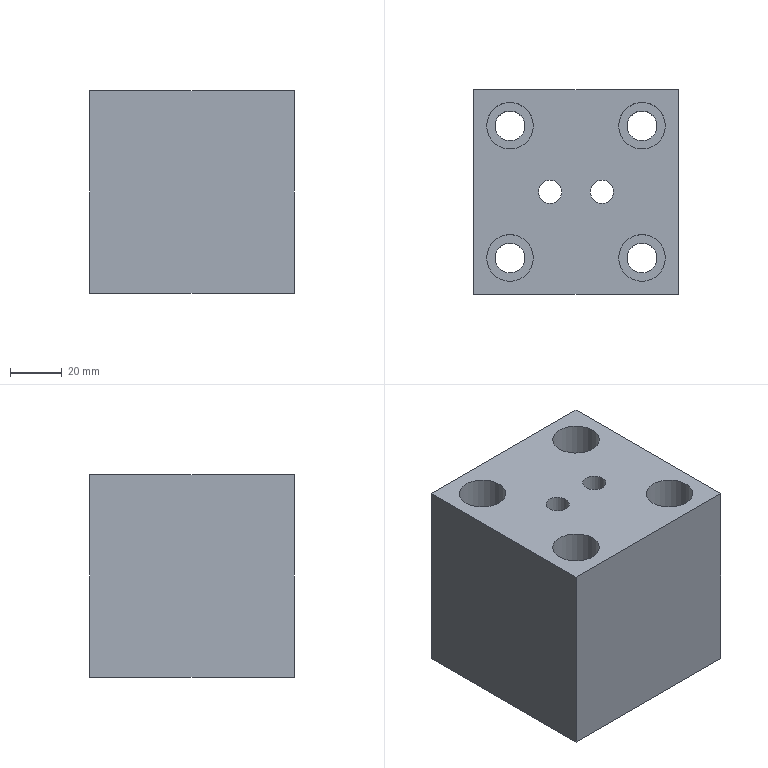Part | STEP file | lll_id4366_x_t | 1 solid | 24 faces | box 79 x 79 x 78 mm | volume 421284 mm3 | plane 12 | cylinder 12 | commonest cylinder face diameters 11.509 x4 18.008 x4 9 x2 14 x2
STEP:
#1=CARTESIAN_POINT('',(2491.255,144.5,-370.));
#2=VERTEX_POINT('',#1);
#3=CARTESIAN_POINT('',(2485.5,144.5,-370.));
#4=DIRECTION('',(0.,0.,1.));
#5=DIRECTION('',(1.,0.,0.));
#6=AXIS2_PLACEMENT_3D('',#3,#4,#5);
#7=CIRCLE('',#6,5.755);
#8=EDGE_CURVE('',#2,#2,#7,.T.);
#9=ORIENTED_EDGE('',*,*,#8,.T.);
#10=EDGE_LOOP('',(#9));
#11=FACE_BOUND('',#10,.T.);
#12=CARTESIAN_POINT('',(2491.255,195.5,-370.));
#13=VERTEX_POINT('',#12);
#14=CARTESIAN_POINT('',(2485.5,195.5,-370.));
#15=DIRECTION('',(0.,0.,1.));
#16=DIRECTION('',(1.,0.,0.));
#17=AXIS2_PLACEMENT_3D('',#14,#15,#16);
#18=CIRCLE('',#17,5.755);
#19=EDGE_CURVE('',#13,#13,#18,.T.);
#20=ORIENTED_EDGE('',*,*,#19,.T.);
#21=EDGE_LOOP('',(#20));
#22=FACE_BOUND('',#21,.T.);
#23=CARTESIAN_POINT('',(2440.255,144.5,-370.));
#24=VERTEX_POINT('',#23);
#25=CARTESIAN_POINT('',(2434.5,144.5,-370.));
#26=DIRECTION('',(0.,0.,1.));
#27=DIRECTION('',(1.,0.,0.));
#28=AXIS2_PLACEMENT_3D('',#25,#26,#27);
#29=CIRCLE('',#28,5.755);
#30=EDGE_CURVE('',#24,#24,#29,.T.);
#31=ORIENTED_EDGE('',*,*,#30,.T.);
#32=EDGE_LOOP('',(#31));
#33=FACE_BOUND('',#32,.T.);
#34=CARTESIAN_POINT('',(2440.255,195.5,-370.));
#35=VERTEX_POINT('',#34);
#36=CARTESIAN_POINT('',(2434.5,195.5,-370.));
#37=DIRECTION('',(0.,0.,1.));
#38=DIRECTION('',(1.,0.,0.));
#39=AXIS2_PLACEMENT_3D('',#36,#37,#38);
#40=CIRCLE('',#39,5.755);
#41=EDGE_CURVE('',#35,#35,#40,.T.);
#42=ORIENTED_EDGE('',*,*,#41,.T.);
#43=EDGE_LOOP('',(#42));
#44=FACE_BOUND('',#43,.T.);
#45=CARTESIAN_POINT('',(2499.5,130.5,-370.));
#46=VERTEX_POINT('',#45);
#47=CARTESIAN_POINT('',(2499.5,209.5,-370.));
#48=VERTEX_POINT('',#47);
#49=CARTESIAN_POINT('',(2499.5,477.5,-370.));
#50=DIRECTION('',(0.,1.,0.));
#51=VECTOR('',#50,1.);
#52=LINE('',#49,#51);
#53=EDGE_CURVE('',#46,#48,#52,.T.);
#54=ORIENTED_EDGE('',*,*,#53,.F.);
#55=CARTESIAN_POINT('',(2420.5,130.5,-370.));
#56=VERTEX_POINT('',#55);
#57=CARTESIAN_POINT('',(2460.,130.5,-370.));
#58=DIRECTION('',(-1.,0.,0.));
#59=VECTOR('',#58,1.);
#60=LINE('',#57,#59);
#61=EDGE_CURVE('',#46,#56,#60,.T.);
#62=ORIENTED_EDGE('',*,*,#61,.T.);
#63=CARTESIAN_POINT('',(2420.5,209.5,-370.));
#64=VERTEX_POINT('',#63);
#65=CARTESIAN_POINT('',(2420.5,477.5,-370.));
#66=DIRECTION('',(0.,-1.,0.));
#67=VECTOR('',#66,1.);
#68=LINE('',#65,#67);
#69=EDGE_CURVE('',#64,#56,#68,.T.);
#70=ORIENTED_EDGE('',*,*,#69,.F.);
#71=CARTESIAN_POINT('',(3042.,209.5,-370.));
#72=DIRECTION('',(-1.,0.,0.));
#73=VECTOR('',#72,1.);
#74=LINE('',#71,#73);
#75=EDGE_CURVE('',#48,#64,#74,.T.);
#76=ORIENTED_EDGE('',*,*,#75,.F.);
#77=EDGE_LOOP('',(#54,#62,#70,#76));
#78=FACE_BOUND('',#77,.T.);
#79=CARTESIAN_POINT('',(2477.,170.,-370.));
#80=VERTEX_POINT('',#79);
#81=CARTESIAN_POINT('',(2470.,170.,-370.));
#82=DIRECTION('',(0.,0.,1.));
#83=DIRECTION('',(1.,0.,0.));
#84=AXIS2_PLACEMENT_3D('',#81,#82,#83);
#85=CIRCLE('',#84,7.);
#86=EDGE_CURVE('',#80,#80,#85,.T.);
#87=ORIENTED_EDGE('',*,*,#86,.T.);
#88=EDGE_LOOP('',(#87));
#89=FACE_BOUND('',#88,.T.);
#90=CARTESIAN_POINT('',(2457.,170.,-370.));
#91=VERTEX_POINT('',#90);
#92=CARTESIAN_POINT('',(2450.,170.,-370.));
#93=DIRECTION('',(0.,0.,-1.));
#94=DIRECTION('',(1.,0.,0.));
#95=AXIS2_PLACEMENT_3D('',#92,#93,#94);
#96=CIRCLE('',#95,7.);
#97=EDGE_CURVE('',#91,#91,#96,.T.);
#98=ORIENTED_EDGE('',*,*,#97,.F.);
#99=EDGE_LOOP('',(#98));
#100=FACE_BOUND('',#99,.T.);
#101=CARTESIAN_POINT('',(3042.,477.5,-370.));
#102=DIRECTION('',(0.,0.,1.));
#103=DIRECTION('',(1.,0.,0.));
#104=AXIS2_PLACEMENT_3D('',#101,#102,#103);
#105=PLANE('',#104);
#106=ADVANCED_FACE('',(#11,#22,#33,#44,#78,#89,#100),#105,.F.);
#107=CARTESIAN_POINT('',(2445.5,170.,-292.));
#108=VERTEX_POINT('',#107);
#109=CARTESIAN_POINT('',(2450.,170.,-292.));
#110=DIRECTION('',(0.,0.,-1.));
#111=DIRECTION('',(-1.,0.,0.));
#112=AXIS2_PLACEMENT_3D('',#109,#110,#111);
#113=CIRCLE('',#112,4.5);
#114=EDGE_CURVE('',#108,#108,#113,.T.);
#115=ORIENTED_EDGE('',*,*,#114,.F.);
#116=EDGE_LOOP('',(#115));
#117=FACE_BOUND('',#116,.T.);
#118=CARTESIAN_POINT('',(2445.5,170.,-302.));
#119=VERTEX_POINT('',#118);
#120=CARTESIAN_POINT('',(2450.,170.,-302.));
#121=DIRECTION('',(0.,0.,-1.));
#122=DIRECTION('',(-1.,0.,0.));
#123=AXIS2_PLACEMENT_3D('',#120,#121,#122);
#124=CIRCLE('',#123,4.5);
#125=EDGE_CURVE('',#119,#119,#124,.T.);
#126=ORIENTED_EDGE('',*,*,#125,.T.);
#127=EDGE_LOOP('',(#126));
#128=FACE_BOUND('',#127,.T.);
#129=CARTESIAN_POINT('',(2450.,170.,-512.));
#130=DIRECTION('',(0.,0.,1.));
#131=DIRECTION('',(1.,0.,0.));
#132=AXIS2_PLACEMENT_3D('',#129,#130,#131);
#133=CYLINDRICAL_SURFACE('',#132,4.5);
#134=ADVANCED_FACE('',(#117,#128),#133,.F.);
#135=ORIENTED_EDGE('',*,*,#114,.T.);
#136=EDGE_LOOP('',(#135));
#137=FACE_BOUND('',#136,.T.);
#138=CARTESIAN_POINT('',(2499.5,209.5,-292.));
#139=VERTEX_POINT('',#138);
#140=CARTESIAN_POINT('',(2499.5,130.5,-292.));
#141=VERTEX_POINT('',#140);
#142=CARTESIAN_POINT('',(2499.5,390.,-292.));
#143=DIRECTION('',(0.,-1.,0.));
#144=VECTOR('',#143,1.);
#145=LINE('',#142,#144);
#146=EDGE_CURVE('',#139,#141,#145,.T.);
#147=ORIENTED_EDGE('',*,*,#146,.F.);
#148=CARTESIAN_POINT('',(2420.5,209.5,-292.));
#149=VERTEX_POINT('',#148);
#150=CARTESIAN_POINT('',(2460.,209.5,-292.));
#151=DIRECTION('',(-1.,0.,0.));
#152=VECTOR('',#151,1.);
#153=LINE('',#150,#152);
#154=EDGE_CURVE('',#139,#149,#153,.T.);
#155=ORIENTED_EDGE('',*,*,#154,.T.);
#156=CARTESIAN_POINT('',(2420.5,130.5,-292.));
#157=VERTEX_POINT('',#156);
#158=CARTESIAN_POINT('',(2420.5,390.,-292.));
#159=DIRECTION('',(0.,1.,0.));
#160=VECTOR('',#159,1.);
#161=LINE('',#158,#160);
#162=EDGE_CURVE('',#157,#149,#161,.T.);
#163=ORIENTED_EDGE('',*,*,#162,.F.);
#164=CARTESIAN_POINT('',(2460.,130.5,-292.));
#165=DIRECTION('',(1.,0.,0.));
#166=VECTOR('',#165,1.);
#167=LINE('',#164,#166);
#168=EDGE_CURVE('',#157,#141,#167,.T.);
#169=ORIENTED_EDGE('',*,*,#168,.T.);
#170=EDGE_LOOP('',(#147,#155,#163,#169));
#171=FACE_BOUND('',#170,.T.);
#172=CARTESIAN_POINT('',(2425.496,195.5,-292.));
#173=VERTEX_POINT('',#172);
#174=CARTESIAN_POINT('',(2434.5,195.5,-292.));
#175=DIRECTION('',(0.,0.,-1.));
#176=DIRECTION('',(-1.,0.,0.));
#177=AXIS2_PLACEMENT_3D('',#174,#175,#176);
#178=CIRCLE('',#177,9.004);
#179=EDGE_CURVE('',#173,#173,#178,.T.);
#180=ORIENTED_EDGE('',*,*,#179,.T.);
#181=EDGE_LOOP('',(#180));
#182=FACE_BOUND('',#181,.T.);
#183=CARTESIAN_POINT('',(2425.496,144.5,-292.));
#184=VERTEX_POINT('',#183);
#185=CARTESIAN_POINT('',(2434.5,144.5,-292.));
#186=DIRECTION('',(0.,0.,-1.));
#187=DIRECTION('',(-1.,0.,0.));
#188=AXIS2_PLACEMENT_3D('',#185,#186,#187);
#189=CIRCLE('',#188,9.004);
#190=EDGE_CURVE('',#184,#184,#189,.T.);
#191=ORIENTED_EDGE('',*,*,#190,.T.);
#192=EDGE_LOOP('',(#191));
#193=FACE_BOUND('',#192,.T.);
#194=CARTESIAN_POINT('',(2476.496,195.5,-292.));
#195=VERTEX_POINT('',#194);
#196=CARTESIAN_POINT('',(2485.5,195.5,-292.));
#197=DIRECTION('',(0.,0.,-1.));
#198=DIRECTION('',(-1.,0.,0.));
#199=AXIS2_PLACEMENT_3D('',#196,#197,#198);
#200=CIRCLE('',#199,9.004);
#201=EDGE_CURVE('',#195,#195,#200,.T.);
#202=ORIENTED_EDGE('',*,*,#201,.T.);
#203=EDGE_LOOP('',(#202));
#204=FACE_BOUND('',#203,.T.);
#205=CARTESIAN_POINT('',(2476.496,144.5,-292.));
#206=VERTEX_POINT('',#205);
#207=CARTESIAN_POINT('',(2485.5,144.5,-292.));
#208=DIRECTION('',(0.,0.,-1.));
#209=DIRECTION('',(-1.,0.,0.));
#210=AXIS2_PLACEMENT_3D('',#207,#208,#209);
#211=CIRCLE('',#210,9.004);
#212=EDGE_CURVE('',#206,#206,#211,.T.);
#213=ORIENTED_EDGE('',*,*,#212,.T.);
#214=EDGE_LOOP('',(#213));
#215=FACE_BOUND('',#214,.T.);
#216=CARTESIAN_POINT('',(2465.5,170.,-292.));
#217=VERTEX_POINT('',#216);
#218=CARTESIAN_POINT('',(2470.,170.,-292.));
#219=DIRECTION('',(0.,0.,1.));
#220=DIRECTION('',(-1.,0.,0.));
#221=AXIS2_PLACEMENT_3D('',#218,#219,#220);
#222=CIRCLE('',#221,4.5);
#223=EDGE_CURVE('',#217,#217,#222,.T.);
#224=ORIENTED_EDGE('',*,*,#223,.F.);
#225=EDGE_LOOP('',(#224));
#226=FACE_BOUND('',#225,.T.);
#227=CARTESIAN_POINT('',(2159.2,390.,-292.));
#228=DIRECTION('',(0.,0.,-1.));
#229=DIRECTION('',(-1.,0.,0.));
#230=AXIS2_PLACEMENT_3D('',#227,#228,#229);
#231=PLANE('',#230);
#232=ADVANCED_FACE('',(#137,#171,#182,#193,#204,#215,#226),#231,.F.);
#233=ORIENTED_EDGE('',*,*,#53,.T.);
#234=CARTESIAN_POINT('',(2499.5,209.5,-289.));
#235=DIRECTION('',(0.,0.,1.));
#236=VECTOR('',#235,1.);
#237=LINE('',#234,#236);
#238=EDGE_CURVE('',#48,#139,#237,.T.);
#239=ORIENTED_EDGE('',*,*,#238,.T.);
#240=ORIENTED_EDGE('',*,*,#146,.T.);
#241=CARTESIAN_POINT('',(2499.5,130.5,-289.));
#242=DIRECTION('',(0.,0.,1.));
#243=VECTOR('',#242,1.);
#244=LINE('',#241,#243);
#245=EDGE_CURVE('',#46,#141,#244,.T.);
#246=ORIENTED_EDGE('',*,*,#245,.F.);
#247=EDGE_LOOP('',(#233,#239,#240,#246));
#248=FACE_OUTER_BOUND('',#247,.T.);
#249=CARTESIAN_POINT('',(2499.5,170.,-289.));
#250=DIRECTION('',(1.,0.,0.));
#251=DIRECTION('',(0.,0.,-1.));
#252=AXIS2_PLACEMENT_3D('',#249,#250,#251);
#253=PLANE('',#252);
#254=ADVANCED_FACE('',(#248),#253,.T.);
#255=ORIENTED_EDGE('',*,*,#61,.F.);
#256=ORIENTED_EDGE('',*,*,#245,.T.);
#257=ORIENTED_EDGE('',*,*,#168,.F.);
#258=CARTESIAN_POINT('',(2420.5,130.5,-289.));
#259=DIRECTION('',(0.,0.,1.));
#260=VECTOR('',#259,1.);
#261=LINE('',#258,#260);
#262=EDGE_CURVE('',#56,#157,#261,.T.);
#263=ORIENTED_EDGE('',*,*,#262,.F.);
#264=EDGE_LOOP('',(#255,#256,#257,#263));
#265=FACE_OUTER_BOUND('',#264,.T.);
#266=CARTESIAN_POINT('',(2460.,130.5,-289.));
#267=DIRECTION('',(0.,-1.,0.));
#268=DIRECTION('',(0.,0.,-1.));
#269=AXIS2_PLACEMENT_3D('',#266,#267,#268);
#270=PLANE('',#269);
#271=ADVANCED_FACE('',(#265),#270,.T.);
#272=ORIENTED_EDGE('',*,*,#69,.T.);
#273=ORIENTED_EDGE('',*,*,#262,.T.);
#274=ORIENTED_EDGE('',*,*,#162,.T.);
#275=CARTESIAN_POINT('',(2420.5,209.5,-289.));
#276=DIRECTION('',(0.,0.,1.));
#277=VECTOR('',#276,1.);
#278=LINE('',#275,#277);
#279=EDGE_CURVE('',#64,#149,#278,.T.);
#280=ORIENTED_EDGE('',*,*,#279,.F.);
#281=EDGE_LOOP('',(#272,#273,#274,#280));
#282=FACE_OUTER_BOUND('',#281,.T.);
#283=CARTESIAN_POINT('',(2420.5,170.,-289.));
#284=DIRECTION('',(-1.,0.,0.));
#285=DIRECTION('',(0.,0.,1.));
#286=AXIS2_PLACEMENT_3D('',#283,#284,#285);
#287=PLANE('',#286);
#288=ADVANCED_FACE('',(#282),#287,.T.);
#289=ORIENTED_EDGE('',*,*,#75,.T.);
#290=ORIENTED_EDGE('',*,*,#279,.T.);
#291=ORIENTED_EDGE('',*,*,#154,.F.);
#292=ORIENTED_EDGE('',*,*,#238,.F.);
#293=EDGE_LOOP('',(#289,#290,#291,#292));
#294=FACE_OUTER_BOUND('',#293,.T.);
#295=CARTESIAN_POINT('',(2460.,209.5,-289.));
#296=DIRECTION('',(0.,1.,0.));
#297=DIRECTION('',(0.,0.,1.));
#298=AXIS2_PLACEMENT_3D('',#295,#296,#297);
#299=PLANE('',#298);
#300=ADVANCED_FACE('',(#294),#299,.T.);
#301=CARTESIAN_POINT('',(2428.745,195.5,-310.));
#302=VERTEX_POINT('',#301);
#303=CARTESIAN_POINT('',(2434.5,195.5,-310.));
#304=DIRECTION('',(0.,0.,-1.));
#305=DIRECTION('',(-1.,0.,0.));
#306=AXIS2_PLACEMENT_3D('',#303,#304,#305);
#307=CIRCLE('',#306,5.755);
#308=EDGE_CURVE('',#302,#302,#307,.T.);
#309=ORIENTED_EDGE('',*,*,#308,.F.);
#310=EDGE_LOOP('',(#309));
#311=FACE_BOUND('',#310,.T.);
#312=ORIENTED_EDGE('',*,*,#41,.F.);
#313=EDGE_LOOP('',(#312));
#314=FACE_BOUND('',#313,.T.);
#315=CARTESIAN_POINT('',(2434.5,195.5,-295.));
#316=DIRECTION('',(0.,0.,-1.));
#317=DIRECTION('',(1.,0.,0.));
#318=AXIS2_PLACEMENT_3D('',#315,#316,#317);
#319=CYLINDRICAL_SURFACE('',#318,5.755);
#320=ADVANCED_FACE('',(#311,#314),#319,.F.);
#321=ORIENTED_EDGE('',*,*,#308,.T.);
#322=EDGE_LOOP('',(#321));
#323=FACE_BOUND('',#322,.T.);
#324=CARTESIAN_POINT('',(2443.504,195.5,-310.));
#325=VERTEX_POINT('',#324);
#326=CARTESIAN_POINT('',(2434.5,195.5,-310.));
#327=DIRECTION('',(0.,0.,-1.));
#328=DIRECTION('',(1.,0.,0.));
#329=AXIS2_PLACEMENT_3D('',#326,#327,#328);
#330=CIRCLE('',#329,9.004);
#331=EDGE_CURVE('',#325,#325,#330,.T.);
#332=ORIENTED_EDGE('',*,*,#331,.F.);
#333=EDGE_LOOP('',(#332));
#334=FACE_BOUND('',#333,.T.);
#335=CARTESIAN_POINT('',(2434.5,195.5,-310.));
#336=DIRECTION('',(0.,0.,-1.));
#337=DIRECTION('',(-1.,0.,0.));
#338=AXIS2_PLACEMENT_3D('',#335,#336,#337);
#339=PLANE('',#338);
#340=ADVANCED_FACE('',(#323,#334),#339,.F.);
#341=ORIENTED_EDGE('',*,*,#331,.T.);
#342=EDGE_LOOP('',(#341));
#343=FACE_BOUND('',#342,.T.);
#344=ORIENTED_EDGE('',*,*,#179,.F.);
#345=EDGE_LOOP('',(#344));
#346=FACE_BOUND('',#345,.T.);
#347=CARTESIAN_POINT('',(2434.5,195.5,-297.));
#348=DIRECTION('',(0.,0.,-1.));
#349=DIRECTION('',(1.,0.,0.));
#350=AXIS2_PLACEMENT_3D('',#347,#348,#349);
#351=CYLINDRICAL_SURFACE('',#350,9.004);
#352=ADVANCED_FACE('',(#343,#346),#351,.F.);
#353=CARTESIAN_POINT('',(2428.745,144.5,-310.));
#354=VERTEX_POINT('',#353);
#355=CARTESIAN_POINT('',(2434.5,144.5,-310.));
#356=DIRECTION('',(0.,0.,-1.));
#357=DIRECTION('',(-1.,0.,0.));
#358=AXIS2_PLACEMENT_3D('',#355,#356,#357);
#359=CIRCLE('',#358,5.755);
#360=EDGE_CURVE('',#354,#354,#359,.T.);
#361=ORIENTED_EDGE('',*,*,#360,.F.);
#362=EDGE_LOOP('',(#361));
#363=FACE_BOUND('',#362,.T.);
#364=ORIENTED_EDGE('',*,*,#30,.F.);
#365=EDGE_LOOP('',(#364));
#366=FACE_BOUND('',#365,.T.);
#367=CARTESIAN_POINT('',(2434.5,144.5,-295.));
#368=DIRECTION('',(0.,0.,-1.));
#369=DIRECTION('',(1.,0.,0.));
#370=AXIS2_PLACEMENT_3D('',#367,#368,#369);
#371=CYLINDRICAL_SURFACE('',#370,5.755);
#372=ADVANCED_FACE('',(#363,#366),#371,.F.);
#373=ORIENTED_EDGE('',*,*,#360,.T.);
#374=EDGE_LOOP('',(#373));
#375=FACE_BOUND('',#374,.T.);
#376=CARTESIAN_POINT('',(2443.504,144.5,-310.));
#377=VERTEX_POINT('',#376);
#378=CARTESIAN_POINT('',(2434.5,144.5,-310.));
#379=DIRECTION('',(0.,0.,-1.));
#380=DIRECTION('',(1.,0.,0.));
#381=AXIS2_PLACEMENT_3D('',#378,#379,#380);
#382=CIRCLE('',#381,9.004);
#383=EDGE_CURVE('',#377,#377,#382,.T.);
#384=ORIENTED_EDGE('',*,*,#383,.F.);
#385=EDGE_LOOP('',(#384));
#386=FACE_BOUND('',#385,.T.);
#387=CARTESIAN_POINT('',(2434.5,144.5,-310.));
#388=DIRECTION('',(0.,0.,-1.));
#389=DIRECTION('',(-1.,0.,0.));
#390=AXIS2_PLACEMENT_3D('',#387,#388,#389);
#391=PLANE('',#390);
#392=ADVANCED_FACE('',(#375,#386),#391,.F.);
#393=ORIENTED_EDGE('',*,*,#383,.T.);
#394=EDGE_LOOP('',(#393));
#395=FACE_BOUND('',#394,.T.);
#396=ORIENTED_EDGE('',*,*,#190,.F.);
#397=EDGE_LOOP('',(#396));
#398=FACE_BOUND('',#397,.T.);
#399=CARTESIAN_POINT('',(2434.5,144.5,-297.));
#400=DIRECTION('',(0.,0.,-1.));
#401=DIRECTION('',(1.,0.,0.));
#402=AXIS2_PLACEMENT_3D('',#399,#400,#401);
#403=CYLINDRICAL_SURFACE('',#402,9.004);
#404=ADVANCED_FACE('',(#395,#398),#403,.F.);
#405=CARTESIAN_POINT('',(2479.745,195.5,-310.));
#406=VERTEX_POINT('',#405);
#407=CARTESIAN_POINT('',(2485.5,195.5,-310.));
#408=DIRECTION('',(0.,0.,-1.));
#409=DIRECTION('',(-1.,0.,0.));
#410=AXIS2_PLACEMENT_3D('',#407,#408,#409);
#411=CIRCLE('',#410,5.755);
#412=EDGE_CURVE('',#406,#406,#411,.T.);
#413=ORIENTED_EDGE('',*,*,#412,.F.);
#414=EDGE_LOOP('',(#413));
#415=FACE_BOUND('',#414,.T.);
#416=ORIENTED_EDGE('',*,*,#19,.F.);
#417=EDGE_LOOP('',(#416));
#418=FACE_BOUND('',#417,.T.);
#419=CARTESIAN_POINT('',(2485.5,195.5,-295.));
#420=DIRECTION('',(0.,0.,-1.));
#421=DIRECTION('',(1.,0.,0.));
#422=AXIS2_PLACEMENT_3D('',#419,#420,#421);
#423=CYLINDRICAL_SURFACE('',#422,5.755);
#424=ADVANCED_FACE('',(#415,#418),#423,.F.);
#425=ORIENTED_EDGE('',*,*,#412,.T.);
#426=EDGE_LOOP('',(#425));
#427=FACE_BOUND('',#426,.T.);
#428=CARTESIAN_POINT('',(2494.504,195.5,-310.));
#429=VERTEX_POINT('',#428);
#430=CARTESIAN_POINT('',(2485.5,195.5,-310.));
#431=DIRECTION('',(0.,0.,-1.));
#432=DIRECTION('',(1.,0.,0.));
#433=AXIS2_PLACEMENT_3D('',#430,#431,#432);
#434=CIRCLE('',#433,9.004);
#435=EDGE_CURVE('',#429,#429,#434,.T.);
#436=ORIENTED_EDGE('',*,*,#435,.F.);
#437=EDGE_LOOP('',(#436));
#438=FACE_BOUND('',#437,.T.);
#439=CARTESIAN_POINT('',(2485.5,195.5,-310.));
#440=DIRECTION('',(0.,0.,-1.));
#441=DIRECTION('',(-1.,0.,0.));
#442=AXIS2_PLACEMENT_3D('',#439,#440,#441);
#443=PLANE('',#442);
#444=ADVANCED_FACE('',(#427,#438),#443,.F.);
#445=ORIENTED_EDGE('',*,*,#435,.T.);
#446=EDGE_LOOP('',(#445));
#447=FACE_BOUND('',#446,.T.);
#448=ORIENTED_EDGE('',*,*,#201,.F.);
#449=EDGE_LOOP('',(#448));
#450=FACE_BOUND('',#449,.T.);
#451=CARTESIAN_POINT('',(2485.5,195.5,-297.));
#452=DIRECTION('',(0.,0.,-1.));
#453=DIRECTION('',(1.,0.,0.));
#454=AXIS2_PLACEMENT_3D('',#451,#452,#453);
#455=CYLINDRICAL_SURFACE('',#454,9.004);
#456=ADVANCED_FACE('',(#447,#450),#455,.F.);
#457=CARTESIAN_POINT('',(2479.745,144.5,-310.));
#458=VERTEX_POINT('',#457);
#459=CARTESIAN_POINT('',(2485.5,144.5,-310.));
#460=DIRECTION('',(0.,0.,-1.));
#461=DIRECTION('',(-1.,0.,0.));
#462=AXIS2_PLACEMENT_3D('',#459,#460,#461);
#463=CIRCLE('',#462,5.755);
#464=EDGE_CURVE('',#458,#458,#463,.T.);
#465=ORIENTED_EDGE('',*,*,#464,.F.);
#466=EDGE_LOOP('',(#465));
#467=FACE_BOUND('',#466,.T.);
#468=ORIENTED_EDGE('',*,*,#8,.F.);
#469=EDGE_LOOP('',(#468));
#470=FACE_BOUND('',#469,.T.);
#471=CARTESIAN_POINT('',(2485.5,144.5,-295.));
#472=DIRECTION('',(0.,0.,-1.));
#473=DIRECTION('',(1.,0.,0.));
#474=AXIS2_PLACEMENT_3D('',#471,#472,#473);
#475=CYLINDRICAL_SURFACE('',#474,5.755);
#476=ADVANCED_FACE('',(#467,#470),#475,.F.);
#477=ORIENTED_EDGE('',*,*,#464,.T.);
#478=EDGE_LOOP('',(#477));
#479=FACE_BOUND('',#478,.T.);
#480=CARTESIAN_POINT('',(2494.504,144.5,-310.));
#481=VERTEX_POINT('',#480);
#482=CARTESIAN_POINT('',(2485.5,144.5,-310.));
#483=DIRECTION('',(0.,0.,-1.));
#484=DIRECTION('',(1.,0.,0.));
#485=AXIS2_PLACEMENT_3D('',#482,#483,#484);
#486=CIRCLE('',#485,9.004);
#487=EDGE_CURVE('',#481,#481,#486,.T.);
#488=ORIENTED_EDGE('',*,*,#487,.F.);
#489=EDGE_LOOP('',(#488));
#490=FACE_BOUND('',#489,.T.);
#491=CARTESIAN_POINT('',(2485.5,144.5,-310.));
#492=DIRECTION('',(0.,0.,-1.));
#493=DIRECTION('',(-1.,0.,0.));
#494=AXIS2_PLACEMENT_3D('',#491,#492,#493);
#495=PLANE('',#494);
#496=ADVANCED_FACE('',(#479,#490),#495,.F.);
#497=ORIENTED_EDGE('',*,*,#487,.T.);
#498=EDGE_LOOP('',(#497));
#499=FACE_BOUND('',#498,.T.);
#500=ORIENTED_EDGE('',*,*,#212,.F.);
#501=EDGE_LOOP('',(#500));
#502=FACE_BOUND('',#501,.T.);
#503=CARTESIAN_POINT('',(2485.5,144.5,-297.));
#504=DIRECTION('',(0.,0.,-1.));
#505=DIRECTION('',(1.,0.,0.));
#506=AXIS2_PLACEMENT_3D('',#503,#504,#505);
#507=CYLINDRICAL_SURFACE('',#506,9.004);
#508=ADVANCED_FACE('',(#499,#502),#507,.F.);
#509=CARTESIAN_POINT('',(2474.5,170.,-302.));
#510=VERTEX_POINT('',#509);
#511=CARTESIAN_POINT('',(2470.,170.,-302.));
#512=DIRECTION('',(0.,0.,-1.));
#513=DIRECTION('',(1.,0.,0.));
#514=AXIS2_PLACEMENT_3D('',#511,#512,#513);
#515=CIRCLE('',#514,4.5);
#516=EDGE_CURVE('',#510,#510,#515,.T.);
#517=ORIENTED_EDGE('',*,*,#516,.T.);
#518=EDGE_LOOP('',(#517));
#519=FACE_BOUND('',#518,.T.);
#520=ORIENTED_EDGE('',*,*,#223,.T.);
#521=EDGE_LOOP('',(#520));
#522=FACE_BOUND('',#521,.T.);
#523=CARTESIAN_POINT('',(2470.,170.,-314.));
#524=DIRECTION('',(0.,0.,1.));
#525=DIRECTION('',(1.,0.,0.));
#526=AXIS2_PLACEMENT_3D('',#523,#524,#525);
#527=CYLINDRICAL_SURFACE('',#526,4.5);
#528=ADVANCED_FACE('',(#519,#522),#527,.F.);
#529=CARTESIAN_POINT('',(2477.,170.,-302.));
#530=VERTEX_POINT('',#529);
#531=CARTESIAN_POINT('',(2470.,170.,-302.));
#532=DIRECTION('',(0.,0.,-1.));
#533=DIRECTION('',(1.,0.,0.));
#534=AXIS2_PLACEMENT_3D('',#531,#532,#533);
#535=CIRCLE('',#534,7.);
#536=EDGE_CURVE('',#530,#530,#535,.T.);
#537=ORIENTED_EDGE('',*,*,#536,.F.);
#538=EDGE_LOOP('',(#537));
#539=FACE_BOUND('',#538,.T.);
#540=ORIENTED_EDGE('',*,*,#86,.F.);
#541=EDGE_LOOP('',(#540));
#542=FACE_BOUND('',#541,.T.);
#543=CARTESIAN_POINT('',(2470.,170.,-512.));
#544=DIRECTION('',(0.,0.,1.));
#545=DIRECTION('',(1.,0.,0.));
#546=AXIS2_PLACEMENT_3D('',#543,#544,#545);
#547=CYLINDRICAL_SURFACE('',#546,7.);
#548=ADVANCED_FACE('',(#539,#542),#547,.F.);
#549=ORIENTED_EDGE('',*,*,#536,.T.);
#550=EDGE_LOOP('',(#549));
#551=FACE_BOUND('',#550,.T.);
#552=ORIENTED_EDGE('',*,*,#516,.F.);
#553=EDGE_LOOP('',(#552));
#554=FACE_BOUND('',#553,.T.);
#555=CARTESIAN_POINT('',(2470.,170.,-302.));
#556=DIRECTION('',(0.,0.,1.));
#557=DIRECTION('',(1.,0.,0.));
#558=AXIS2_PLACEMENT_3D('',#555,#556,#557);
#559=PLANE('',#558);
#560=ADVANCED_FACE('',(#551,#554),#559,.F.);
#561=CARTESIAN_POINT('',(2443.,170.,-302.));
#562=VERTEX_POINT('',#561);
#563=CARTESIAN_POINT('',(2450.,170.,-302.));
#564=DIRECTION('',(0.,0.,1.));
#565=DIRECTION('',(-1.,0.,0.));
#566=AXIS2_PLACEMENT_3D('',#563,#564,#565);
#567=CIRCLE('',#566,7.);
#568=EDGE_CURVE('',#562,#562,#567,.T.);
#569=ORIENTED_EDGE('',*,*,#568,.T.);
#570=EDGE_LOOP('',(#569));
#571=FACE_BOUND('',#570,.T.);
#572=ORIENTED_EDGE('',*,*,#97,.T.);
#573=EDGE_LOOP('',(#572));
#574=FACE_BOUND('',#573,.T.);
#575=CARTESIAN_POINT('',(2450.,170.,-512.));
#576=DIRECTION('',(0.,0.,1.));
#577=DIRECTION('',(1.,0.,0.));
#578=AXIS2_PLACEMENT_3D('',#575,#576,#577);
#579=CYLINDRICAL_SURFACE('',#578,7.);
#580=ADVANCED_FACE('',(#571,#574),#579,.F.);
#581=ORIENTED_EDGE('',*,*,#125,.F.);
#582=EDGE_LOOP('',(#581));
#583=FACE_BOUND('',#582,.T.);
#584=ORIENTED_EDGE('',*,*,#568,.F.);
#585=EDGE_LOOP('',(#584));
#586=FACE_BOUND('',#585,.T.);
#587=CARTESIAN_POINT('',(2450.,170.,-302.));
#588=DIRECTION('',(0.,0.,-1.));
#589=DIRECTION('',(-1.,0.,0.));
#590=AXIS2_PLACEMENT_3D('',#587,#588,#589);
#591=PLANE('',#590);
#592=ADVANCED_FACE('',(#583,#586),#591,.T.);
#593=CLOSED_SHELL('',(#106,#134,#232,#254,#271,#288,#300,#320,#340,#352,#372,#392,#404,#424,#444,#456,#476,#496,#508,#528,#548,#560,#580,#592));
#594=MANIFOLD_SOLID_BREP('',#593);
#595=(LENGTH_UNIT()NAMED_UNIT(*)SI_UNIT(.MILLI.,.METRE.));
#596=UNCERTAINTY_MEASURE_WITH_UNIT(LENGTH_MEASURE(0.00002),#595,'','');
#597=(NAMED_UNIT(*)PLANE_ANGLE_UNIT()SI_UNIT($,.RADIAN.));
#598=PLANE_ANGLE_MEASURE_WITH_UNIT(PLANE_ANGLE_MEASURE(0.01745),#597);
#599=DIMENSIONAL_EXPONENTS(0.,0.,0.,0.,0.,0.,0.);
#600=(CONVERSION_BASED_UNIT('DEGREE',#598)NAMED_UNIT(#599)PLANE_ANGLE_UNIT());
#601=(NAMED_UNIT(*)SI_UNIT($,.STERADIAN.)SOLID_ANGLE_UNIT());
#602=(GEOMETRIC_REPRESENTATION_CONTEXT(3)GLOBAL_UNCERTAINTY_ASSIGNED_CONTEXT((#596))GLOBAL_UNIT_ASSIGNED_CONTEXT((#595,#600,#601))REPRESENTATION_CONTEXT('',''));
#603=ADVANCED_BREP_SHAPE_REPRESENTATION('',(#594),#602);